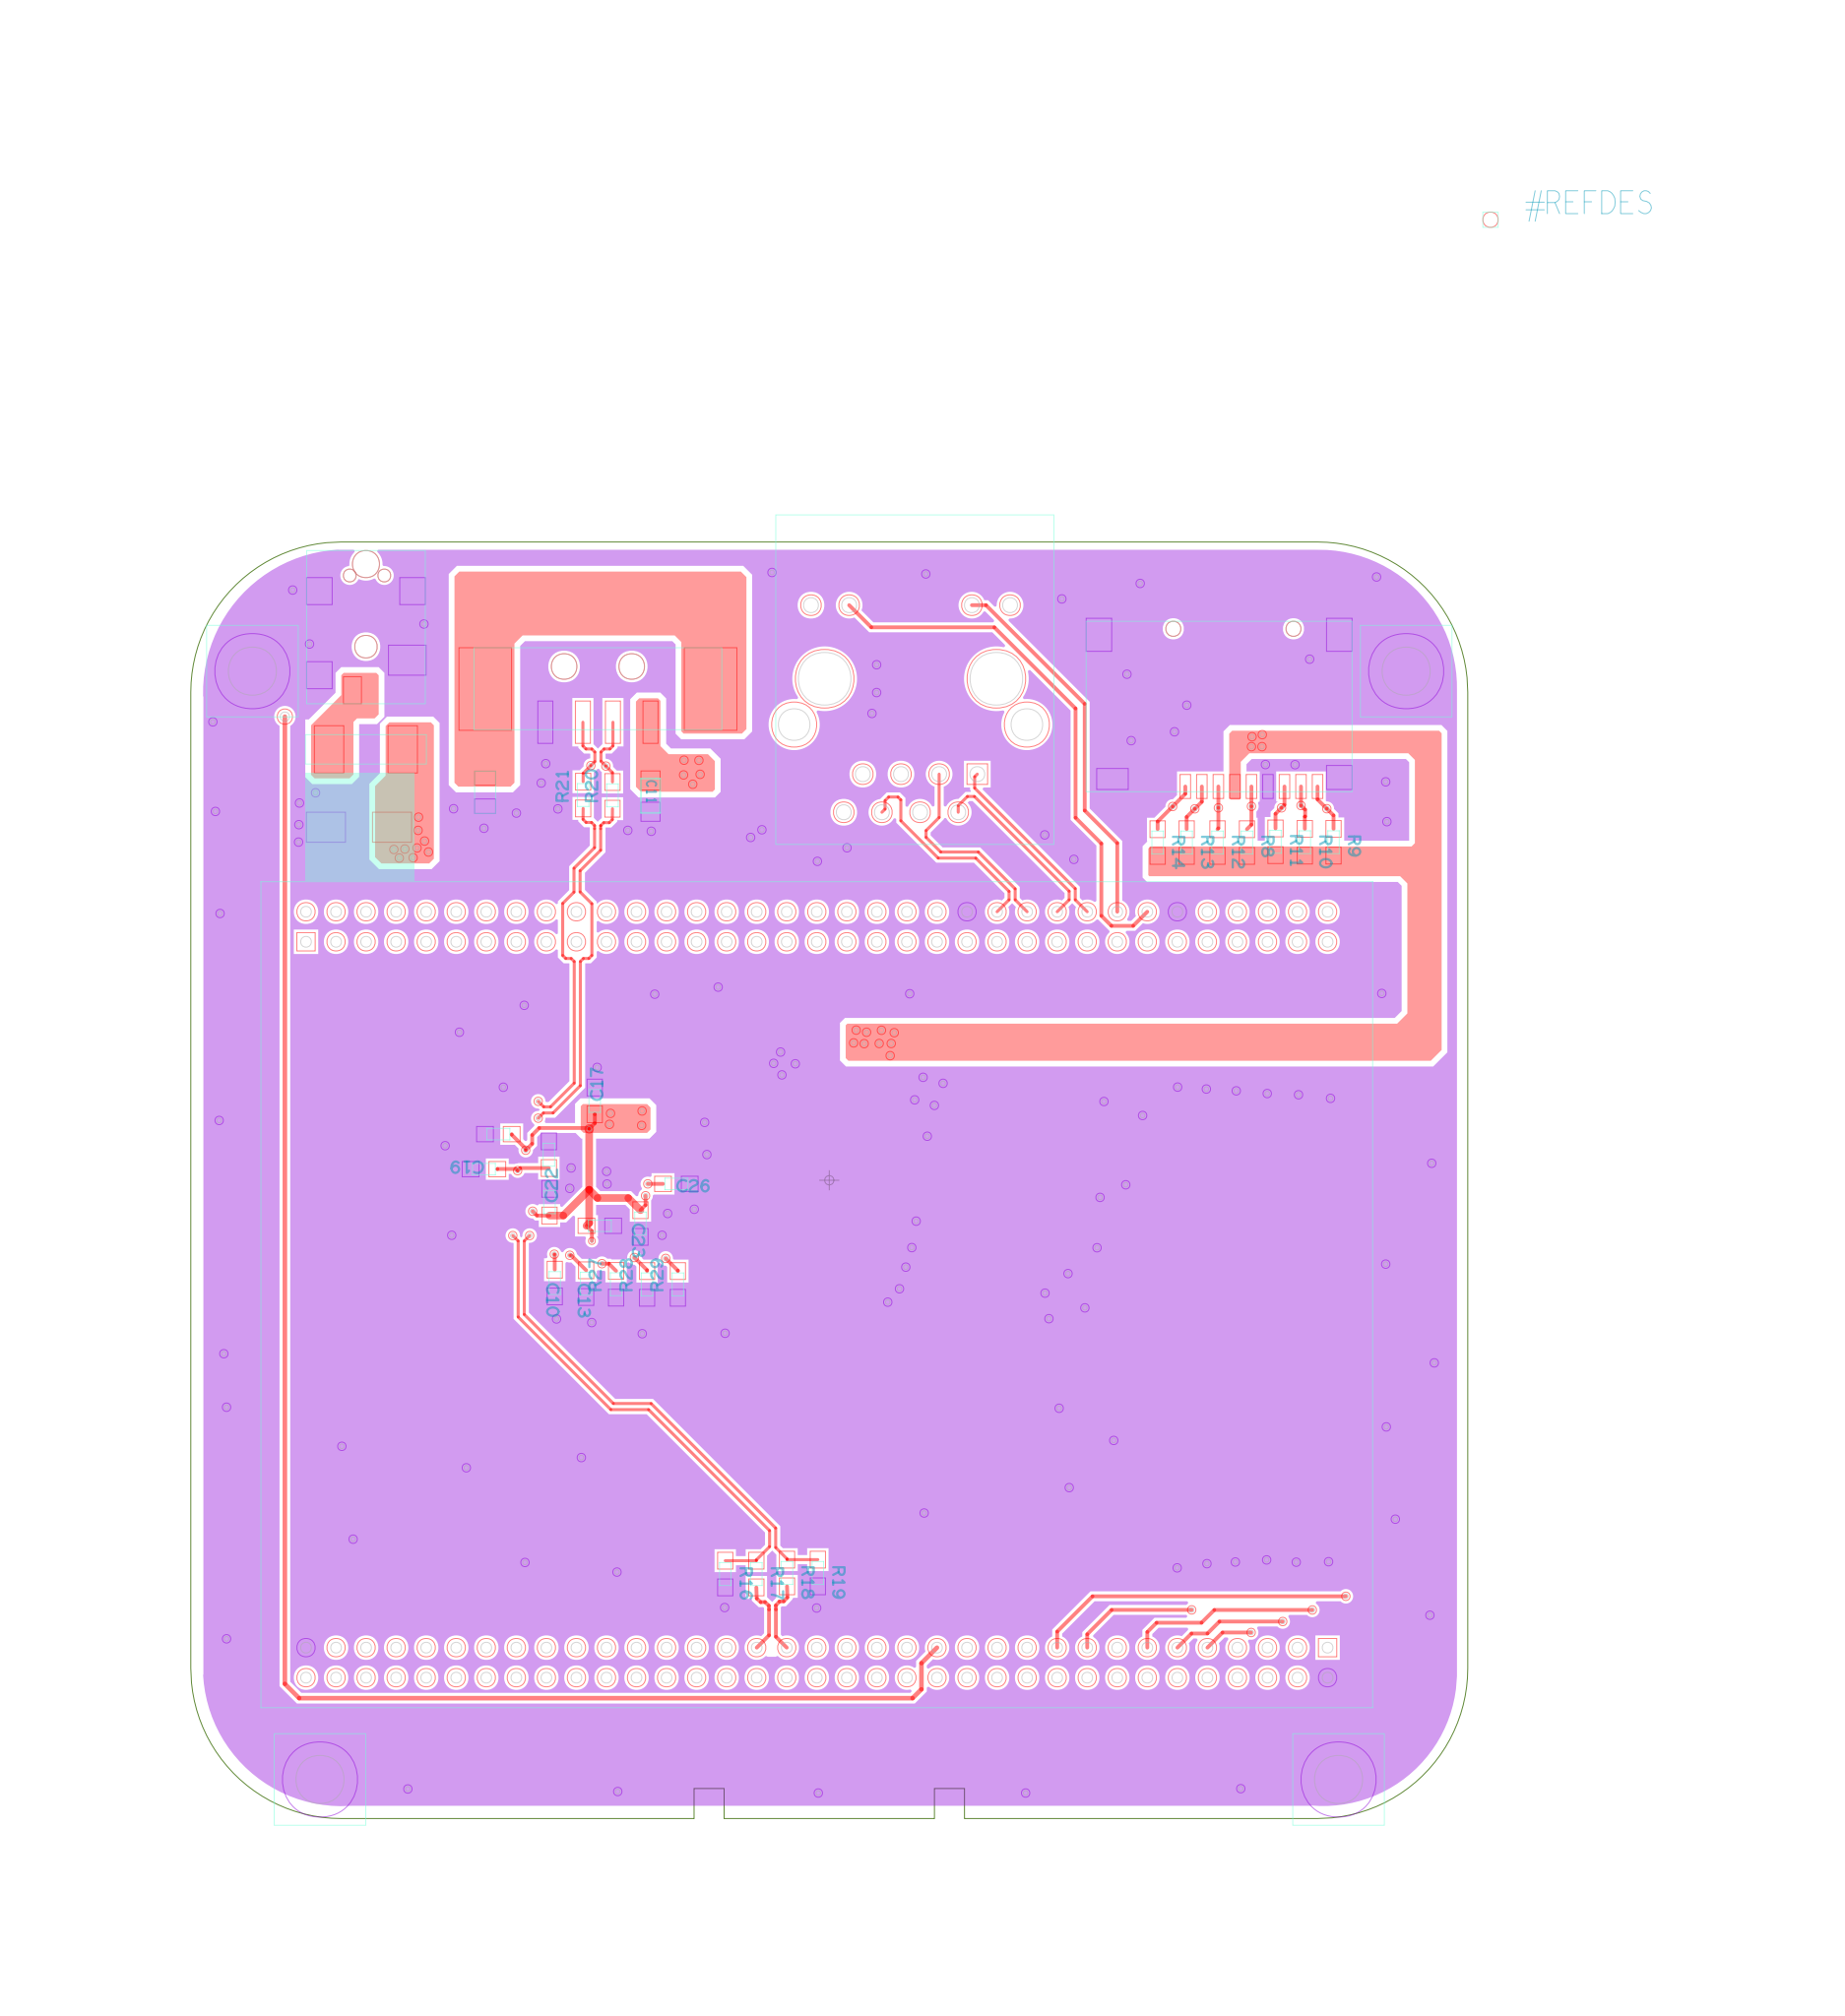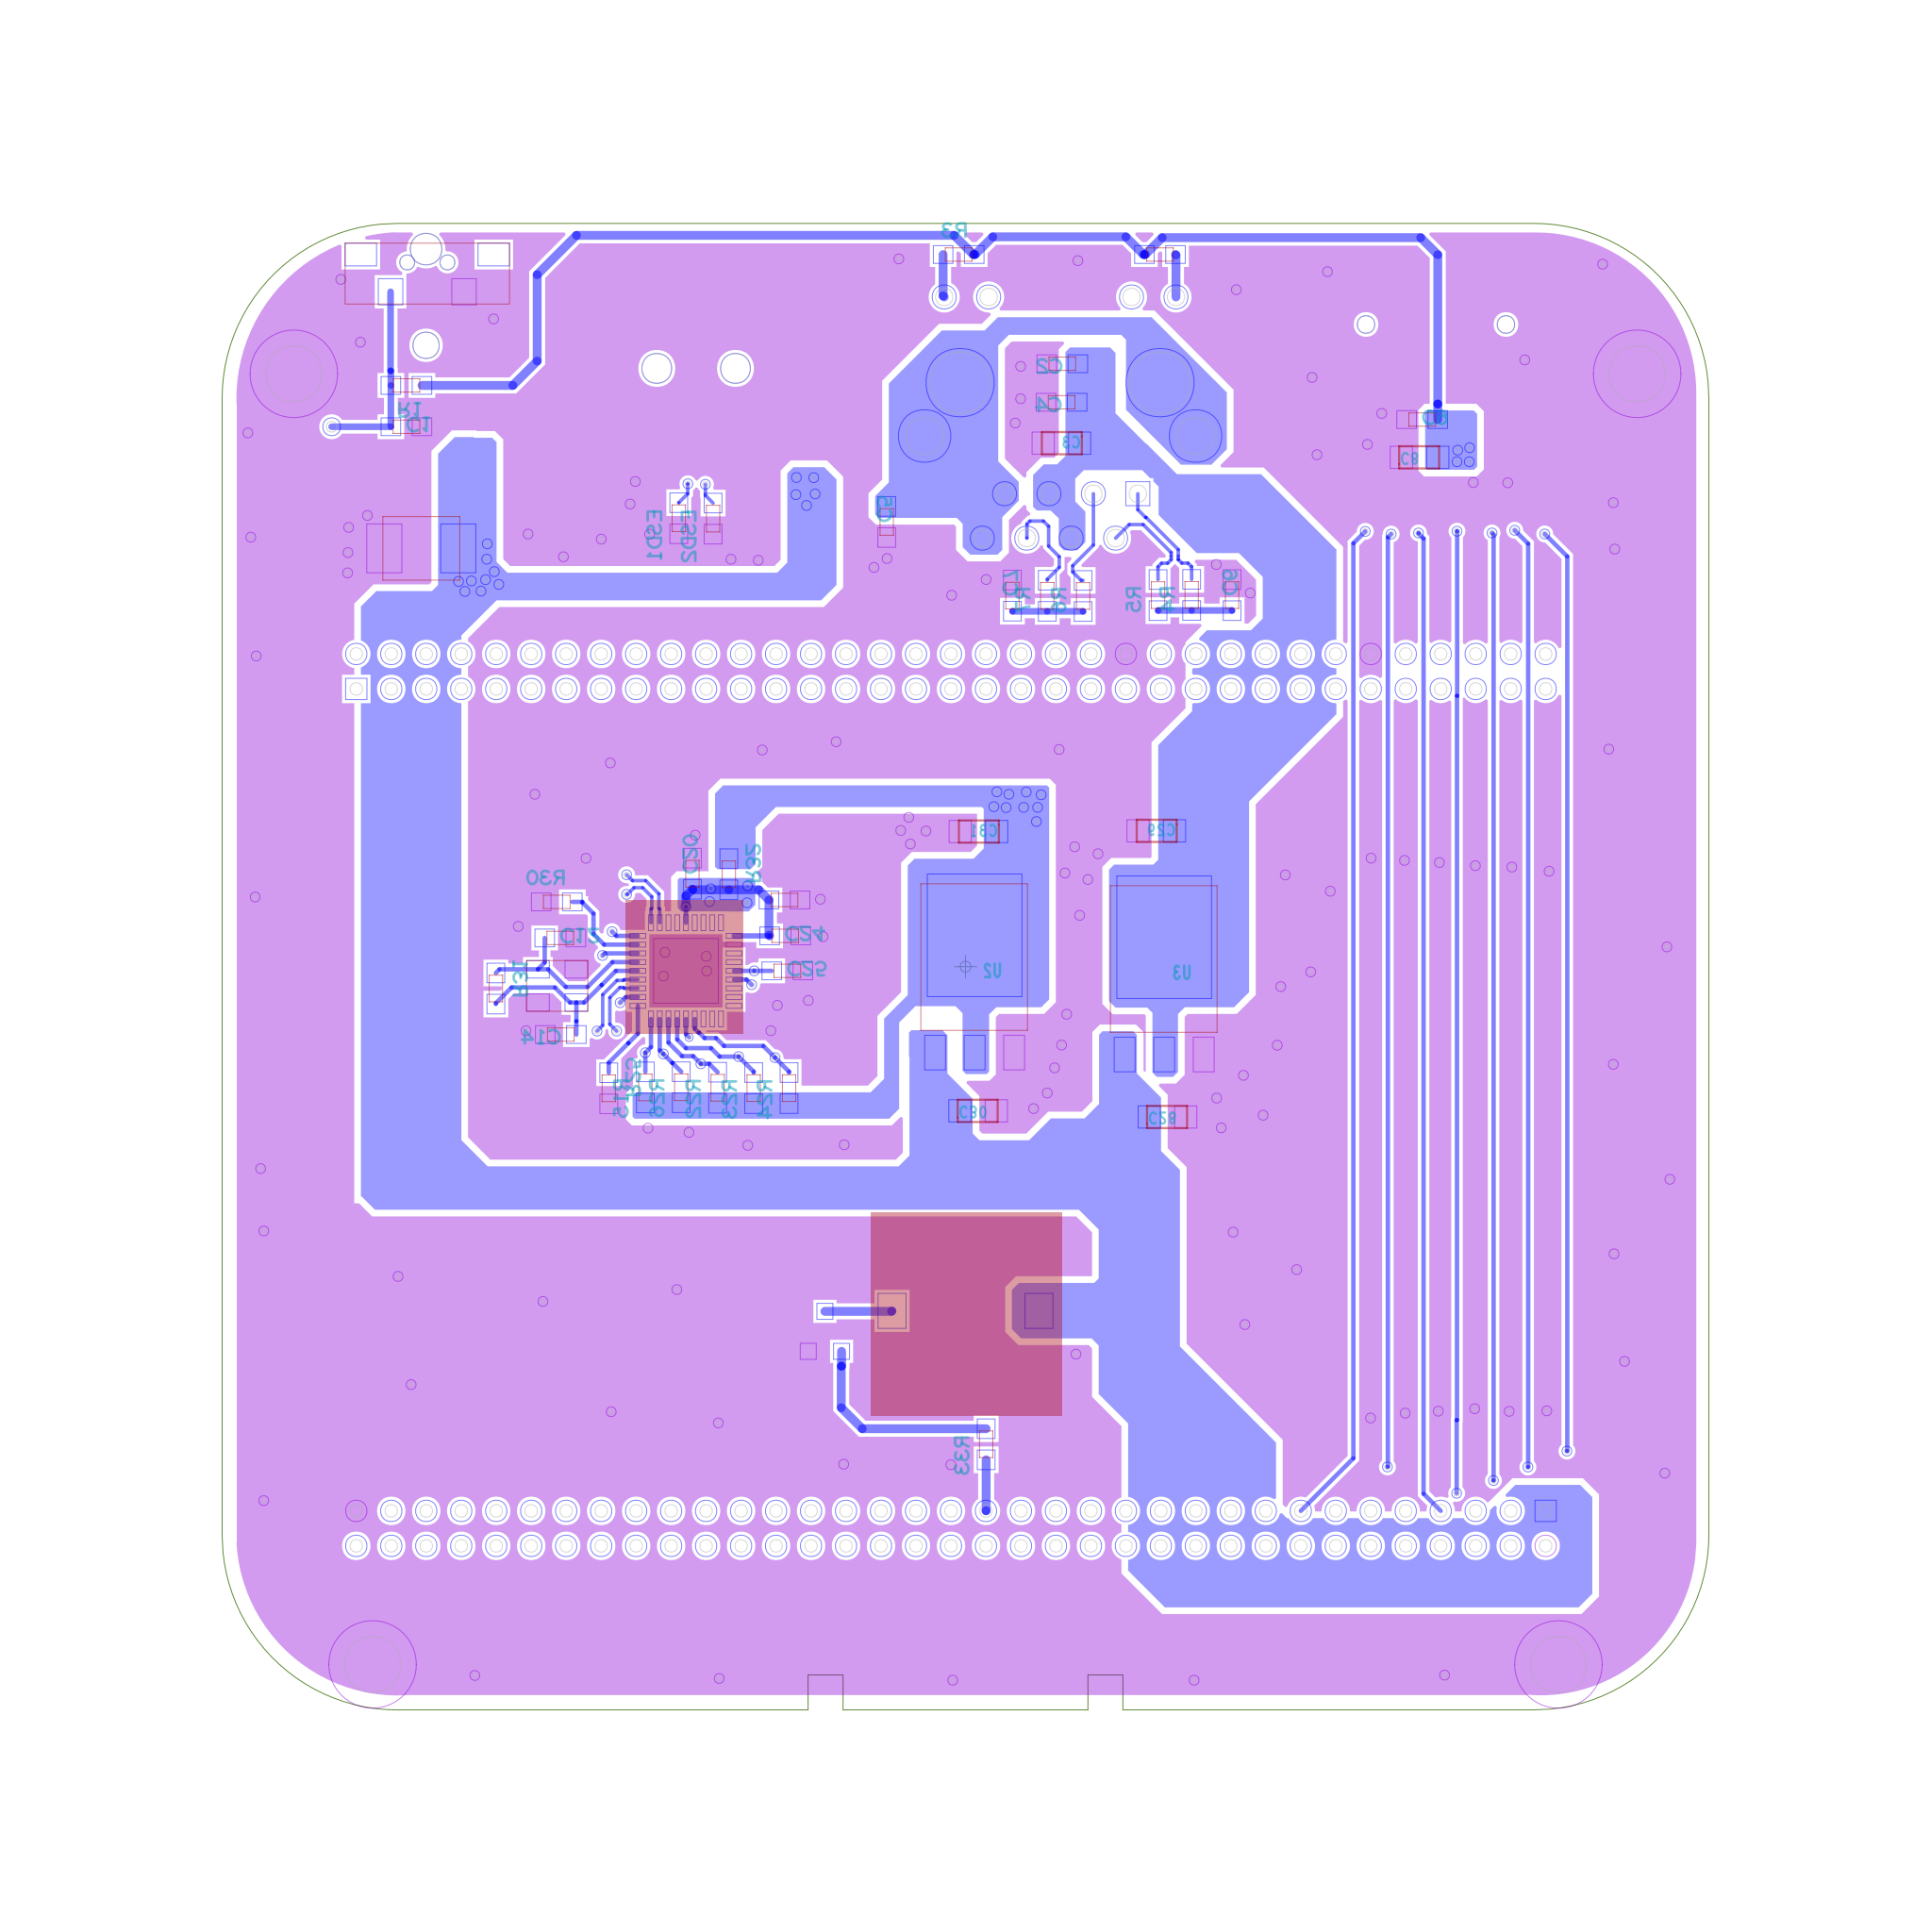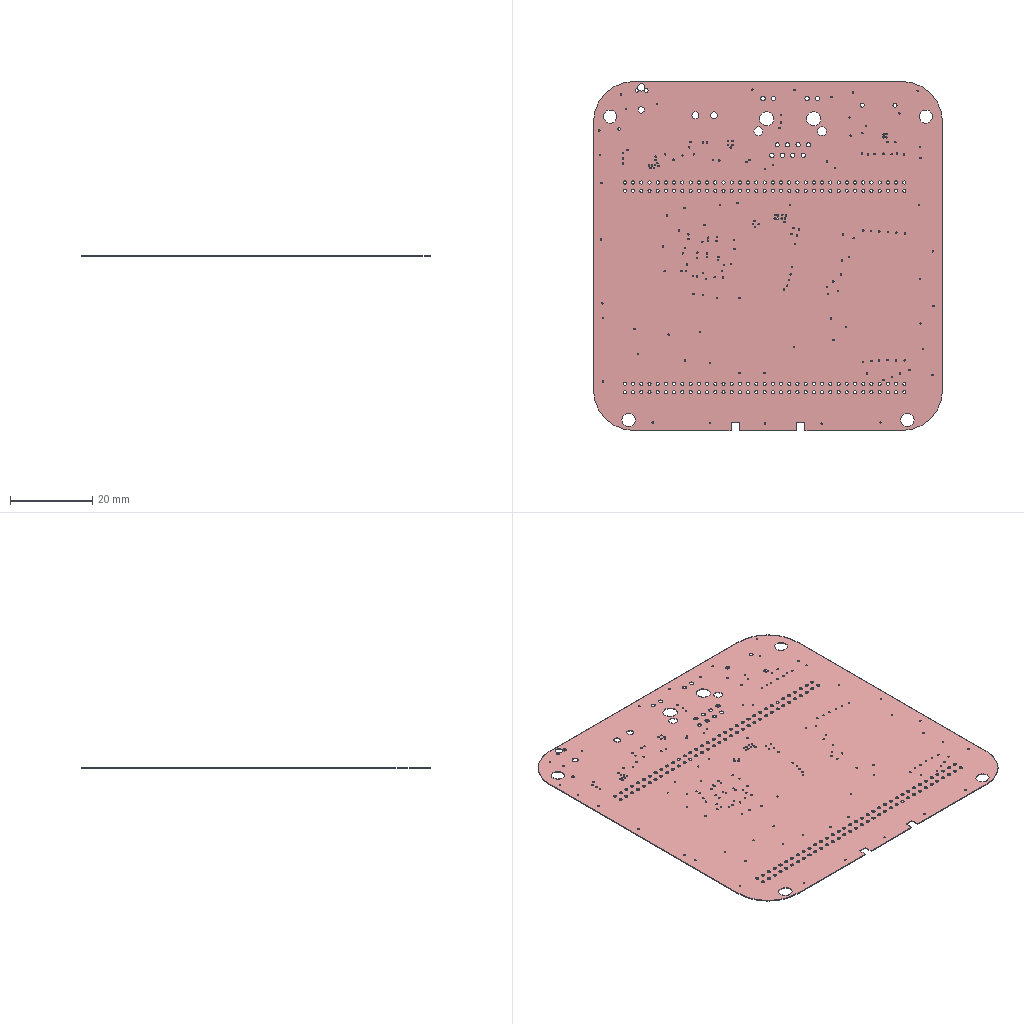Circuit board layout | Cadence Allegro | box 85 x 85 x 0.2 mm
Layer stack:
# Cadence Allegro layer stack of  (unit mm; from the constraint file cross-section; dielectric type: 0 not recorded (Allegro does not mark core vs prepreg), 3 surface material)
index,name,kind,layer,copper_thickness_mm,dielectric_type,dielectric_thickness_mm,dielectric_material,dielectric_constant
0,Top Surface,other,,,,,,
1,TOP,copper,TOP,0.0305,,,,
2,Dielectric1,dielectric,,,0,0.2032,FR-4,4.5
3,BOTTOM,copper,BOTTOM,0.0305,,,,
4,Bottom Surface,other,,,,,,
# drill layer pairs: low layer,high layer
drill_pair,TOP,BOTTOM
Part placement:
REFDES,COMP_VALUE,SYM_NAME,SYM_X,SYM_Y,SYM_ROTATE,SYM_MIRROR
BUZZER1,SPEAKER,FM1,0.000,-775.000,270.000,YES
C1,104,C0603,-1258.436,1215.490,180.000,YES
C2,104,C0603,217.882,1357.330,0.000,YES
C3,10uF,C0805,256.888,1178.454,0.000,YES
C4,104,C0603,216.306,1270.650,0.000,YES
C5,10n,C0603,-177.300,1001.154,270.000,YES
C6,104,C0603,600.061,836.461,270.000,YES
C7,104,C0603,105.591,835.279,270.000,YES
C8,10uF,C0805,981.060,1146.540,180.000,YES
C9,0.1uF,C0603,1027.946,1231.644,180.000,YES
C10,104,C0603,-719.445,-269.496,270.000,NO
C11,10uF,C0805,-468.466,1048.040,270.000,NO
C12,33pF,C0603,-912.110,64.614,180.000,YES
C13,104,C0603,-637.098,-271.071,270.000,NO
C14,33pF,C0603,-910.929,-152.870,0.000,YES
C15,1uF,C0603,-867.194,120.958,180.000,NO
C16,104,C0603,-407.398,150.114,180.000,YES
C17,104,C0603,-614.640,208.032,90.000,NO
C18,1uF,C0603,-734.811,66.980,90.000,NO
C19,104,C0603,-905.018,29.156,180.000,NO
C20,1uF,C0603,-614.641,209.215,270.000,YES
C21,104,C0603,-601.244,-119.382,0.000,NO
C22,104,C0603,-733.232,-57.524,90.000,NO
C23,104,C0603,-494.864,-113.472,270.000,NO
C24,104,C0603,-405.819,69.343,180.000,YES
C25,1uF,C0603,-401.091,-9.457,180.000,YES
C26,104,C0603,-400.697,-9.457,0.000,NO
C27,100u/35V,SMD6,-1232.432,925.506,270.000,NO
C28,10uF,C0805,413.700,-338.446,180.000,YES
C29,10uF,C0805,470.436,305.744,0.000,YES
C30,10uF,C0805,-12.608,-324.656,180.000,YES
C31,10uF,C0805,70.132,304.168,0.000,YES
D1,5.6V,DO-214AA-SMB,-1224.946,941.660,0.000,YES
ESD1,TVS:ULCE0505A015FR,R0603,-645.373,1009.428,90.000,YES
ESD2,TVS:ULCE0505A015FR,R0603,-568.148,1008.640,90.000,YES
F1,5V@2A 1206,F2410,-1214.307,1129.598,0.000,NO
FB1,600R-100M,F0805,-901.866,1017.308,180.000,NO
H1,CON1,MH_125_,-1334.646,-1570.866,0.000,NO
H6,CON1,MH_125_,1334.646,-1570.866,0.000,NO
H11,CON1,MH_125_,-1511.811,1334.646,0.000,NO
H15,CON1,MH_125_,1511.811,1334.646,0.000,NO
J1,HR911105A,HR911105A,212.598,901.417,0.000,NO
J2,DC-041,DC-041,-1214.173,1615.354,270.000,NO
Q1,MMBT3904AL,SOT-23-D,-278.952,-866.012,0.000,YES
R1,10K,R0603,-1258.436,1308.474,180.000,YES
R2,1K,R0603,437.732,1603.185,180.000,YES
R3,1K,R0603,-15.366,1603.185,0.000,YES
R4,51 ,1%,R0603,509.050,836.855,90.000,YES
R5,51R, 1%,R0603,433.400,836.461,90.000,YES
R6,51R ,1%,R0603,264.769,834.492,90.000,YES
R7,51R,1%,R0603,183.997,834.885,90.000,YES
R8,10K,R0603,1094.531,885.319,270.000,NO
R9,10K,R0603,1321.476,886.106,270.000,NO
R10,10K,R0603,1246.220,886.106,270.000,NO
R11,10K,R0603,1169.394,887.287,270.000,NO
R12,10K,R0603,1017.307,885.319,270.000,NO
R13,10K,R0603,936.539,885.319,270.000,NO
R14,10K,R0603,860.496,885.319,270.000,NO
R15,0R,R0603,-720.626,-271.858,90.000,YES
R16,NC,R0603,-272.650,-1032.280,270.000,NO
R17,0R,R0603,-191.091,-1032.280,270.000,NO
R18,0R,R0603,-110.713,-1029.524,270.000,NO
R19,NC,R0603,-29.945,-1029.524,270.000,NO
R20,22R,R0603,-568.148,1009.034,90.000,NO
R21,22R,R0603,-644.979,1009.821,90.000,NO
R22,NC,R0603,-557.906,-272.649,90.000,YES
R23,NC,R0603,-476.740,-273.437,90.000,YES
R24,NC,R0603,-397.154,-273.437,90.000,YES
R25,10K,R0603,-802.972,-273.831,270.000,YES
R26,10K,R0603,-639.854,-271.464,90.000,YES
R27,10K,R0603,-558.693,-272.649,90.000,NO
R28,10K,R0603,-477.528,-273.043,90.000,NO
R29,10K,R0603,-396.760,-273.043,90.000,NO
R30,12K,1%,R0603,-919.988,145.780,0.000,YES
R31,1M,R0603,-1057.102,-49.252,270.000,YES
R32,0R,R0603,-532.688,208.034,270.000,YES
R33,1K,R0603,46.492,-1075.226,90.000,YES
SU1,MICROSD/TF_SLOT,SD,1021.654,1032.283,180.000,NO
SW1,POWON,SMT_TD_15EA,-1211.417,1585.433,0.000,YES
TINY1,4418BV1,TINYPRO,1424.016,782.677,180.000,NO
U1,USB2514B_QFN36_MIN,QFN-36,-629.217,-9.457,90.000,YES
U2,AMS1086CD-3.3,TO-252,109.532,-193.452,0.000,YES
U3,AMS1086CD-1.8,TO-252,536.233,-197.788,0.000,YES
USBH1,USB  A,USB-1001,-606.299,1346.850,180.000,NO
Y1,24MHz,SMD_3225,-850.252,-100.469,0.000,YES
Pad and via stacks:
# Allegro (Cadence) via spans and padstacks; design units: ("mils" 3 1000)
# via spans: padstack,start_layer,end_layer,net_example,count
VIA8-BGA-Q,ETCH/TOP,ETCH/BOTTOM,N9763008,1
VIA12-22BGA,ETCH/TOP,ETCH/BOTTOM,DGND,186
VIA24-Q,ETCH/TOP,ETCH/BOTTOM,N9814926,1
# Allegro padstack definitions: name,start_layer,end_layer,drill,plating,holeType,type
C50D31,"ETCH/TOP","ETCH/BOTTOM",31.0,"PLATED","circle_drill","through"
C5D47NP,"ETCH/TOP","ETCH/BOTTOM",47.0,"PLATED","circle_drill","through"
SMDO98X160,"ETCH/TOP","ETCH/TOP",0.0,"PLATED","none","smd"
SMD44X40,"ETCH/TOP","ETCH/TOP",0.0,"PLATED","none","smd"
SMD50X50-L,"ETCH/TOP","ETCH/TOP",0.0,"PLATED","none","smd"
S21X20,"ETCH/TOP","ETCH/TOP",0.0,"PLATED","none","smd"
REV079X110,"ETCH/TOP","ETCH/TOP",0.0,"PLATED","none","smd"
SMD55X50,"ETCH/TOP","ETCH/TOP",0.0,"NON_PLATED","none","smd"
SMD36X36-L,"ETCH/TOP","ETCH/TOP",0.0,"PLATED","none","smd"
PAD46,"ETCH/TOP","ETCH/TOP",0.0,"NON_PLATED","none","smd"
PAD47,"ETCH/TOP","ETCH/TOP",0.0,"NON_PLATED","none","smd"
PAD4,"ETCH/TOP","ETCH/TOP",0.0,"NON_PLATED","none","smd"
PAD5,"ETCH/TOP","ETCH/TOP",0.0,"NON_PLATED","none","smd"
C5MMD3MM2,"ETCH/TOP","ETCH/BOTTOM",125.98,"PLATED","circle_drill","through"
C54D39,"ETCH/TOP","ETCH/BOTTOM",39.0,"PLATED","circle_drill","through"
S54D39-L-A,"ETCH/TOP","ETCH/BOTTOM",39.0,"PLATED","circle_drill","through"
C118D78,"ETCH/TOP","ETCH/BOTTOM",82.681,"PLATED","circle_drill","through"
C150D137NP,"ETCH/TOP","ETCH/BOTTOM",137.799,"NON_PLATED","circle_drill","through"
PAD12,"ETCH/TOP","ETCH/BOTTOM",59.059,"NON_PLATED","circle_drill","through"
PAD11,"ETCH/TOP","ETCH/BOTTOM",70.87,"NON_PLATED","circle_drill","through"
PAD10,"ETCH/TOP","ETCH/TOP",0.0,"NON_PLATED","none","smd"
PAD9,"ETCH/TOP","ETCH/TOP",0.0,"NON_PLATED","none","smd"
PAD8,"ETCH/TOP","ETCH/TOP",0.0,"NON_PLATED","none","smd"
O1M23X1M05XO0M85X0M65,"ETCH/TOP","ETCH/BOTTOM",25.591,"PLATED","oval slot","through"
SMDR78X78,"ETCH/TOP","ETCH/TOP",0.0,"PLATED","none","smd"
R78X78D33X60,"ETCH/TOP","ETCH/BOTTOM",33.0,"PLATED","oval slot","through"
SMDR16X63,"ETCH/TOP","ETCH/TOP",0.0,"PLATED","none","smd"
SMDR40X48,"ETCH/TOP","ETCH/TOP",0.0,"PLATED","none","smd"
PAD26,"ETCH/TOP","ETCH/BOTTOM",39.37,"NON_PLATED","circle_drill","through"
PAD25,"ETCH/TOP","ETCH/TOP",0.0,"NON_PLATED","none","smd"
PAD24,"ETCH/TOP","ETCH/TOP",0.0,"NON_PLATED","none","smd"
PAD23,"ETCH/TOP","ETCH/TOP",0.0,"NON_PLATED","none","smd"
PAD22,"ETCH/TOP","ETCH/TOP",0.0,"NON_PLATED","none","smd"
C48D28,"ETCH/TOP","ETCH/BOTTOM",28.0,"PLATED","circle_drill","through"
S48D28,"ETCH/TOP","ETCH/BOTTOM",28.0,"PLATED","circle_drill","through"
SMD213X276,"ETCH/TOP","ETCH/TOP",0.0,"PLATED","none","smd"
SMD47X78,"ETCH/TOP","ETCH/TOP",0.0,"PLATED","none","smd"
SMD211X211_TH,"ETCH/TOP","ETCH/TOP",0.0,"PLATED","none","smd"
SMDR28X40,"ETCH/TOP","ETCH/TOP",0.0,"PLATED","none","smd"
SMDO11X35,"ETCH/TOP","ETCH/TOP",0.0,"PLATED","none","smd"
SMDO35X11,"ETCH/TOP","ETCH/TOP",0.0,"PLATED","none","smd"
SMDR176X176,"ETCH/TOP","ETCH/TOP",0.0,"PLATED","none","smd"
SMD65_12,"ETCH/TOP","ETCH/TOP",0.0,"PLATED","none","smd"
F70X65,"ETCH/TOP","ETCH/TOP",0.0,"PLATED","none","smd"
C150D78,"ETCH/TOP","ETCH/BOTTOM",78.74,"PLATED","circle_drill","through"
C65D39,"ETCH/TOP","ETCH/BOTTOM",39.37,"PLATED","circle_drill","through"
C60D39,"ETCH/TOP","ETCH/BOTTOM",39.37,"PLATED","circle_drill","through"
TP,"ETCH/TOP","ETCH/TOP",0.0,"PLATED","none","smd"
PAD44,"ETCH/TOP","ETCH/TOP",0.0,"NON_PLATED","none","smd"
PAD43,"ETCH/TOP","ETCH/TOP",0.0,"NON_PLATED","none","smd"
C54D30,"ETCH/TOP","ETCH/BOTTOM",30.0,"PLATED","circle_drill","through"
SMDO34X10,"ETCH/TOP","ETCH/TOP",0.0,"PLATED","none","smd"
SMDO10X34,"ETCH/TOP","ETCH/TOP",0.0,"PLATED","none","smd"
PAD27,"ETCH/TOP","ETCH/BOTTOM",33.461,"NON_PLATED","circle_drill","through"
PAD29,"ETCH/TOP","ETCH/TOP",0.0,"NON_PLATED","none","smd"
PAD28,"ETCH/TOP","ETCH/TOP",0.0,"NON_PLATED","none","smd"
PAD51,"ETCH/TOP","ETCH/BOTTOM",66.929,"NON_PLATED","circle_drill","through"
PAD50,"ETCH/TOP","ETCH/TOP",0.0,"NON_PLATED","none","smd"
PAD49,"ETCH/TOP","ETCH/TOP",0.0,"NON_PLATED","none","smd"
PAD45,"ETCH/TOP","ETCH/BOTTOM",27.559,"PLATED","circle_drill","through"
Y1,"ETCH/TOP","ETCH/TOP",0.0,"NON_PLATED","none","smd"
PAD19,"ETCH/TOP","ETCH/BOTTOM",35.429,"NON_PLATED","circle_drill","through"
PAD17,"ETCH/TOP","ETCH/TOP",0.0,"NON_PLATED","none","smd"
PAD18,"ETCH/TOP","ETCH/TOP",0.0,"NON_PLATED","none","smd"
PAD16,"ETCH/TOP","ETCH/TOP",0.0,"NON_PLATED","none","smd"
PAD48,"ETCH/TOP","ETCH/BOTTOM",125.984,"PLATED","circle_drill","through"
D0_9X2_7SS0_6OB,"ETCH/TOP","ETCH/BOTTOM",35.433,"PLATED","oval slot","through"
D0_9X2_1SS0_6OB,"ETCH/TOP","ETCH/BOTTOM",35.433,"PLATED","oval slot","through"
S0_28X2_6,"ETCH/TOP","ETCH/TOP",0.0,"NON_PLATED","none","smd"
SMD1_14RE1_27,"ETCH/TOP","ETCH/TOP",0.0,"NON_PLATED","none","smd"
VIA10-BGA,"ETCH/TOP","ETCH/BOTTOM",10.0,"PLATED","circle_drill","through"
VIA16-BGA,"ETCH/TOP","ETCH/BOTTOM",16.0,"PLATED","circle_drill","through"
VIA8-BGA-Q,"ETCH/TOP","ETCH/BOTTOM",8.0,"PLATED","circle_drill","through"
PAD42,"ETCH/TOP","ETCH/TOP",0.0,"NON_PLATED","none","smd"
F26X20,"ETCH/TOP","ETCH/TOP",0.0,"PLATED","none","smd"
VIA24-Q,"ETCH/TOP","ETCH/BOTTOM",24.0,"PLATED","circle_drill","through"
VIA12-22BGA,"ETCH/TOP","ETCH/BOTTOM",12.0,"PLATED","circle_drill","through"
Y8,"ETCH/TOP","ETCH/BOTTOM",31.496,"PLATED","circle_drill","through"
R90X28,"ETCH/TOP","ETCH/TOP",0.0,"PLATED","none","smd"
S37,"ETCH/TOP","ETCH/TOP",0.0,"PLATED","none","smd"
Y6,"ETCH/TOP","ETCH/BOTTOM",33.465,"PLATED","circle_drill","through"
R20X16,"ETCH/TOP","ETCH/TOP",0.0,"PLATED","none","smd"
Design rules, without the lines most boards share, first 16 of 33 lines:
# Cadence Allegro design rules of  (from the Constraint Manager export constraints.dcfx, design unit mil; typed fields in mm)
# columns: name | kind | enabled | priority | scope1 | scope2 | descriptor | typed fields (field=value)
# Allegro precedence (priority 1 wins): 1 Region class-to-class, 2 Region class, 3 Region, 4 class-to-class, 5 DiffPair/Bus/NetGroup override, 6 NetClass, 7 constraint set (CSet) default
# per-layer values are written LAYER=value in the descriptor and LAYER:mm in the typed field; a maximum of 0 means no limit set
# --- net classes (and buses / net groups) ---
90OHM | NetClass | enabled | 6 | N9762804, N9762824, DM1-, DP1+ | All | Net Class (members: 4 Net) |
PWR_PH | NetClass | enabled | 6 | DGND, VDD_5V, N9763008, VDD_1.8V | All | Net Class (members: 4 Net) |
90OHM_PH | NetClass | enabled | 6 | N9762804, N9762824, DM1-, DP1+ | All | Net Class (members: 4 Net) |
# --- track widths, neck and differential-pair gap (physical constraint sets) ---
DEFAULT | PhysicalCSet | enabled | 7 | Design default | All | Physical Constraint (Min Line Width=10mil) (Max Line Width=0mil) (Min Neck Width=8mil) (Max Neck Length=0mil) (DiffPair Primary Gap=8mil) (DiffPair Neck Gap=8mil) (DiffPair Min Space=0mil) (DiffPair Coupled +Tol=0mil) (DiffPair Coupled -Tol=0mil) (Min BB Via Stagger=5mil) (Max BB Via Stagger=0mil) (T-junctions=ANYWHERE) (Pad-pad direct connect=ALL_ALLOWED) (Allowed vias=VIA12-22BGA, VIA10-BGA, VIA16-BGA, VIA8-BGA-Q, VIA24-Q) | min_line_width=0.254 min_neck_width=0.2032 min_bvia_stagger=0.127 max_bvia_stagger=0 ts_allowed=ANYWHERE diffp_primary_gap=0.2032 diffp_neck_gap=0.2032 max_line_width=0 maximum_neck_length=0 pad_pad_direct_connect=ALL_ALLOWED allow_on_etch_subclass=TRUE diffp_coupled_plus=0 diffp_coupled_minus=0 diffp_min_space=0 vias=VIA12-22BGA,VIA10-BGA,VIA16-BGA,VIA8-BGA-Q,VIA24-Q
# --- clearances: line / pad / via / shape / hole (spacing constraint sets) ---
DEFAULT | SpacingCSet | enabled | 7 | Design default | All | Clearance Constraint (Line-Line=8mil) (Line-SMD Pad=8mil) (Line-Thru Pin=8mil) (Line-Via=8mil) (Line-Shape=8mil) (SMD Pad-SMD Pad=5mil) (Thru Pin-Thru Pin=5mil) (Thru Pin-SMD Pad=5mil) (SMD Pad-Via=5mil) (Thru Pin-Via=5mil) (Via-Via=5mil) (Shape-SMD Pad=8mil) (Shape-Thru Pin=8mil) (Shape-Via=8mil) (Shape-Shape=15mil) (Hole-Hole=8mil) (Hole-Line=10mil) (Hole-Shape=8mil) (BB Via-BB Via=5mil) (uVia-uVia=5mil) | thrupin_to_thrupin_spacing=0.127 thrupin_to_smdpin_spacing=0.127 thrupin_to_thruvia_spacing=0.127 line_to_thrupin_spacing=0.2032 thrupin_to_shape_spacing=0.2032 smdpin_to_smdpin_spacing=0.127 smdpin_to_thruvia_spacing=0.127 line_to_smdpin_spacing=0.2032 shape_to_smdpin_spacing=0.2032 thruvia_to_thruvia_spacing=0.127 line_to_thruvia_spacing=0.2032 shape_to_thruvia_spacing=0.2032 line_to_line_spacing=0.2032 line_to_shape_spacing=0.2032 shape_to_shape_spacing=0.381 bbv_to_bbv_spacing=0.127 bbv_to_thrupin_spacing=0.127 bbv_to_smdpin_spacing=0.127 bbv_to_thruvia_spacing=0.127 bbv_to_line_spacing=0.2032 bbv_to_shape_spacing=0.2032 bbv_to_testpin_spacing=0.127 bbv_to_testvia_spacing=0.127 testpin_to_testpin_spacing=0.127 testpin_to_thrupin_spacing=0.127 smdpin_to_testpin_spacing=0.127 testpin_to_thruvia_spacing=0.127 testpin_to_testvia_spacing=0.127 line_to_testpin_spacing=0.2032 shape_to_testpin_spacing=0.2032 testvia_to_testvia_spacing=0.127 testvia_to_thrupin_spacing=0.127 smdpin_to_testvia_spacing=0.127 testvia_to_thruvia_spacing=0.127 line_to_testvia_spacing=0.2032 shape_to_testvia_spacing=0.2032 bondpad_to_bondpad_spacing=0.127 thrupin_to_bondpad_spacing=0.127 smdpin_to_bondpad_spacing=0.127 bondpad_to_thruvia_spacing=0.127 bondpad_to_line_spacing=0.2032 bondpad_to_shape_spacing=0.127 bondpad_to_bbv_spacing=0.127 bondpad_to_testpin_spacing=0.127 bondpad_to_testvia_spacing=0.127 min_bvia_gap=0.127 hole_to_pin_spacing=0.2032 hole_to_via_spacing=0.2032 hole_to_line_spacing=0.254 hole_to_shape_spacing=0.2032 hole_to_hole_spacing=0.2032 mvia_to_mvia_spacing=0.127 mvia_to_thrupin_spacing=0.127 mvia_to_smdpin_spacing=0.127 mvia_to_thruvia_spacing=0.127 mvia_to_bbv_spacing=0.127 mvia_to_line_spacing=0.2032 mvia_to_shape_spacing=0.2032 mvia_to_testpin_spacing=0.127 mvia_to_testvia_spacing=0.127 bondpad_to_mvia_spacing=0.127 bondpad_to_bondpad_diffp_spc=0.127
DEFAULT | SameNetSpacingCSet | disabled (SAME_NET=FALSE) | 7 | Design default | All | Same-Net Clearance (Line-Line=5mil) (Line-SMD Pad=5mil) (Line-Thru Pin=5mil) (Line-Via=5mil) (Line-Shape=5mil) (SMD Pad-SMD Pad=5mil) (Thru Pin-Thru Pin=5mil) (Thru Pin-SMD Pad=5mil) (SMD Pad-Via=5mil) (Thru Pin-Via=5mil) (Via-Via=5mil) (Shape-SMD Pad=5mil) (Shape-Thru Pin=5mil) (Shape-Via=5mil) (Shape-Shape=5mil) (Hole-Hole=8mil) (Hole-Line=8mil) (Hole-Shape=8mil) (BB Via-BB Via=5mil) (uVia-uVia=5mil) | sn_thrupin_to_thrupin_spacing=0.127 sn_thrupin_to_smdpin_spacing=0.127 sn_thrupin_to_thruvia_spacing=0.127 sn_line_to_thrupin_spacing=0.127 sn_thrupin_to_shape_spacing=0.127 sn_smdpin_to_smdpin_spacing=0.127 sn_smdpin_to_thruvia_spacing=0.127 sn_line_to_smdpin_spacing=0.127 sn_shape_to_smdpin_spacing=0.127 sn_thruvia_to_thruvia_spacing=0.127 sn_line_to_thruvia_spacing=0.127 sn_shape_to_thruvia_spacing=0.127 sn_line_to_line_spacing=0.127 sn_line_to_shape_spacing=0.127 sn_shape_to_shape_spacing=0.127 sn_bbv_to_bbv_spacing=0.127 sn_bbv_to_thrupin_spacing=0.127 sn_bbv_to_smdpin_spacing=0.127 sn_bbv_to_thruvia_spacing=0.127 sn_bbv_to_line_spacing=0.127 sn_bbv_to_shape_spacing=0.127 sn_bbv_to_testpin_spacing=0.127 sn_bbv_to_testvia_spacing=0.127 sn_testpin_to_testpin_spacing=0.127 sn_testpin_to_thrupin_spacing=0.127 sn_smdpin_to_testpin_spacing=0.127 sn_testpin_to_thruvia_spacing=0.127 sn_testpin_to_testvia_spacing=0.127 sn_line_to_testpin_spacing=0.127 sn_shape_to_testpin_spacing=0.127 sn_testvia_to_testvia_spacing=0.127 sn_testvia_to_thrupin_spacing=0.127 sn_smdpin_to_testvia_spacing=0.127 sn_testvia_to_thruvia_spacing=0.127 sn_line_to_testvia_spacing=0.127 sn_shape_to_testvia_spacing=0.127 sn_bondpad_to_bondpad_spacing=0.127 sn_thrupin_to_bondpad_spacing=0.127 sn_smdpin_to_bondpad_spacing=0.127 sn_bondpad_to_thruvia_spacing=0.127 sn_bondpad_to_line_spacing=0.127 sn_bondpad_to_shape_spacing=0.127 sn_bondpad_to_bbv_spacing=0.127 sn_bondpad_to_testpin_spacing=0.127 sn_bondpad_to_testvia_spacing=0.127 same_net=FALSE sn_hole_to_pin_spacing=0.2032 sn_hole_to_via_spacing=0.2032 sn_hole_to_line_spacing=0.2032 sn_hole_to_shape_spacing=0.2032 sn_hole_to_hole_spacing=0.2032 sn_mvia_to_mvia_spacing=0.127 sn_mvia_to_thrupin_spacing=0.127 sn_mvia_to_smdpin_spacing=0.127 sn_mvia_to_thruvia_spacing=0.127 sn_mvia_to_bbv_spacing=0.127 sn_mvia_to_line_spacing=0.127 sn_mvia_to_shape_spacing=0.127 sn_mvia_to_testpin_spacing=0.127 sn_mvia_to_testvia_spacing=0.127 sn_bondpad_to_mvia_spacing=0.127
# --- differential pairs (4) ---
DIFFPAIR37 | DiffPair | enabled | 5 | DM1- | DP1+ | Differential Pair (Primary Gap=8mil) (Min Line Width=10mil) (Physical CSet=DEFAULT) | gap=0.2032 width=0.254 electricalcset=CF
DIFFPAIR38 | DiffPair | enabled | 5 | XUHDM | XUHDP | Differential Pair (Primary Gap=8mil) (Min Line Width=10mil) (Physical CSet=DEFAULT) | gap=0.2032 width=0.254 electricalcset=CF